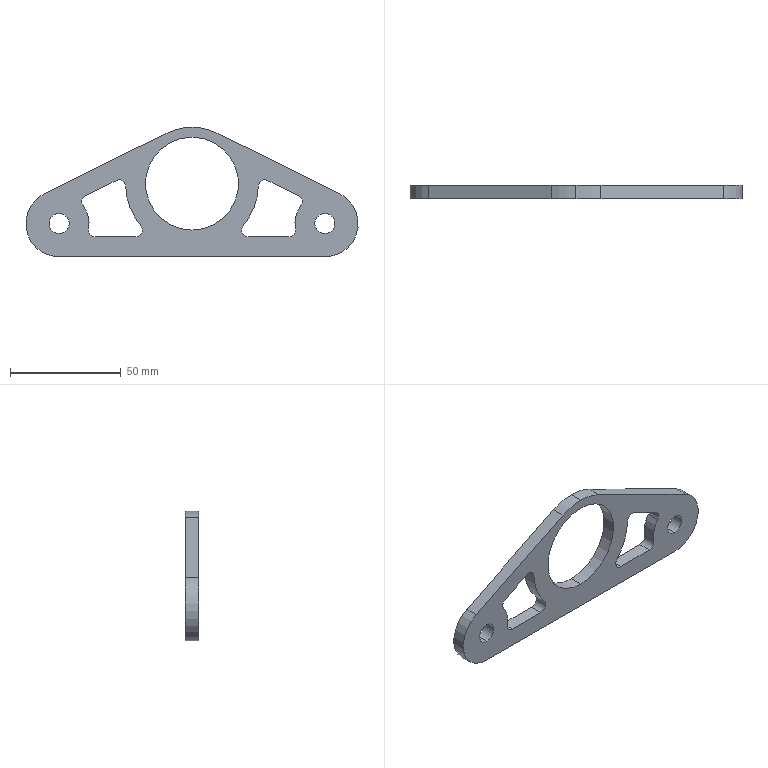Part | STEP file | 2026.6.15-Main Assembly图.sldasm-Part-164 | 1 solid | 33 faces | box 150 x 6 x 58.455 mm | volume 22886 mm3 | cylinder 24 | plane 9 | commonest cylinder face diameters 6 x10 9.06 x4 27.06 x2 30 x2 41.91 x2 50.91 x2
STEP:
#1=CARTESIAN_POINT('',(-1582.519,1443.764,3392.966));
#2=VERTEX_POINT('',#1);
#3=CARTESIAN_POINT('',(-1571.238,1443.764,3395.602));
#4=VERTEX_POINT('',#3);
#5=CARTESIAN_POINT('',(-1571.238,1443.764,3370.147));
#6=DIRECTION('',(0.,1.,0.));
#7=DIRECTION('',(0.,0.,1.));
#8=AXIS2_PLACEMENT_3D('',#5,#6,#7);
#9=CIRCLE('',#8,25.455);
#10=EDGE_CURVE('',#2,#4,#9,.T.);
#11=ORIENTED_EDGE('',*,*,#10,.F.);
#12=CARTESIAN_POINT('',(-1637.886,1443.764,3365.593));
#13=VERTEX_POINT('',#12);
#14=CARTESIAN_POINT('',(-1637.886,1443.764,3365.593));
#15=DIRECTION('',(-0.8964,0.,-0.4432));
#16=VECTOR('',#15,1000.);
#17=LINE('',#14,#16);
#18=EDGE_CURVE('',#2,#13,#17,.T.);
#19=ORIENTED_EDGE('',*,*,#18,.T.);
#20=CARTESIAN_POINT('',(-1631.238,1443.764,3337.147));
#21=VERTEX_POINT('',#20);
#22=CARTESIAN_POINT('',(-1631.238,1443.764,3352.147));
#23=DIRECTION('',(0.,1.,0.));
#24=DIRECTION('',(0.,0.,1.));
#25=AXIS2_PLACEMENT_3D('',#22,#23,#24);
#26=CIRCLE('',#25,15.);
#27=EDGE_CURVE('',#21,#13,#26,.T.);
#28=ORIENTED_EDGE('',*,*,#27,.F.);
#29=CARTESIAN_POINT('',(-1511.238,1443.764,3337.147));
#30=VERTEX_POINT('',#29);
#31=CARTESIAN_POINT('',(-1631.238,1443.764,3337.147));
#32=DIRECTION('',(1.,0.,0.));
#33=VECTOR('',#32,1000.);
#34=LINE('',#31,#33);
#35=EDGE_CURVE('',#21,#30,#34,.T.);
#36=ORIENTED_EDGE('',*,*,#35,.T.);
#37=CARTESIAN_POINT('',(-1504.591,1443.764,3365.593));
#38=VERTEX_POINT('',#37);
#39=CARTESIAN_POINT('',(-1511.238,1443.764,3352.147));
#40=DIRECTION('',(0.,1.,0.));
#41=DIRECTION('',(0.,0.,1.));
#42=AXIS2_PLACEMENT_3D('',#39,#40,#41);
#43=CIRCLE('',#42,15.);
#44=EDGE_CURVE('',#38,#30,#43,.T.);
#45=ORIENTED_EDGE('',*,*,#44,.F.);
#46=CARTESIAN_POINT('',(-1559.957,1443.764,3392.966));
#47=VERTEX_POINT('',#46);
#48=CARTESIAN_POINT('',(-1504.591,1443.764,3365.593));
#49=DIRECTION('',(-0.8964,0.,0.4432));
#50=VECTOR('',#49,1000.);
#51=LINE('',#48,#50);
#52=EDGE_CURVE('',#38,#47,#51,.T.);
#53=ORIENTED_EDGE('',*,*,#52,.T.);
#54=CARTESIAN_POINT('',(-1571.238,1443.764,3370.147));
#55=DIRECTION('',(0.,1.,0.));
#56=DIRECTION('',(0.,0.,1.));
#57=AXIS2_PLACEMENT_3D('',#54,#55,#56);
#58=CIRCLE('',#57,25.455);
#59=EDGE_CURVE('',#4,#47,#58,.T.);
#60=ORIENTED_EDGE('',*,*,#59,.F.);
#61=EDGE_LOOP('',(#11,#19,#28,#36,#45,#53,#60));
#62=FACE_OUTER_BOUND('',#61,.T.);
#63=CARTESIAN_POINT('',(-1631.238,1443.764,3356.677));
#64=VERTEX_POINT('',#63);
#65=CARTESIAN_POINT('',(-1631.238,1443.764,3347.617));
#66=VERTEX_POINT('',#65);
#67=CARTESIAN_POINT('',(-1631.238,1443.764,3352.147));
#68=DIRECTION('',(0.,1.,0.));
#69=DIRECTION('',(0.,0.,1.));
#70=AXIS2_PLACEMENT_3D('',#67,#68,#69);
#71=CIRCLE('',#70,4.53);
#72=EDGE_CURVE('',#64,#66,#71,.T.);
#73=ORIENTED_EDGE('',*,*,#72,.T.);
#74=CARTESIAN_POINT('',(-1631.238,1443.764,3352.147));
#75=DIRECTION('',(0.,1.,0.));
#76=DIRECTION('',(0.,0.,1.));
#77=AXIS2_PLACEMENT_3D('',#74,#75,#76);
#78=CIRCLE('',#77,4.53);
#79=EDGE_CURVE('',#66,#64,#78,.T.);
#80=ORIENTED_EDGE('',*,*,#79,.T.);
#81=EDGE_LOOP('',(#73,#80));
#82=FACE_BOUND('',#81,.T.);
#83=CARTESIAN_POINT('',(-1511.238,1443.764,3356.677));
#84=VERTEX_POINT('',#83);
#85=CARTESIAN_POINT('',(-1511.238,1443.764,3347.617));
#86=VERTEX_POINT('',#85);
#87=CARTESIAN_POINT('',(-1511.238,1443.764,3352.147));
#88=DIRECTION('',(0.,1.,0.));
#89=DIRECTION('',(0.,0.,1.));
#90=AXIS2_PLACEMENT_3D('',#87,#88,#89);
#91=CIRCLE('',#90,4.53);
#92=EDGE_CURVE('',#84,#86,#91,.T.);
#93=ORIENTED_EDGE('',*,*,#92,.T.);
#94=CARTESIAN_POINT('',(-1511.238,1443.764,3352.147));
#95=DIRECTION('',(0.,1.,0.));
#96=DIRECTION('',(0.,0.,1.));
#97=AXIS2_PLACEMENT_3D('',#94,#95,#96);
#98=CIRCLE('',#97,4.53);
#99=EDGE_CURVE('',#86,#84,#98,.T.);
#100=ORIENTED_EDGE('',*,*,#99,.T.);
#101=EDGE_LOOP('',(#93,#100));
#102=FACE_BOUND('',#101,.T.);
#103=CARTESIAN_POINT('',(-1571.238,1443.764,3391.102));
#104=VERTEX_POINT('',#103);
#105=CARTESIAN_POINT('',(-1571.238,1443.764,3349.192));
#106=VERTEX_POINT('',#105);
#107=CARTESIAN_POINT('',(-1571.238,1443.764,3370.147));
#108=DIRECTION('',(0.,1.,0.));
#109=DIRECTION('',(0.,0.,1.));
#110=AXIS2_PLACEMENT_3D('',#107,#108,#109);
#111=CIRCLE('',#110,20.955);
#112=EDGE_CURVE('',#104,#106,#111,.T.);
#113=ORIENTED_EDGE('',*,*,#112,.T.);
#114=CARTESIAN_POINT('',(-1571.238,1443.764,3370.147));
#115=DIRECTION('',(0.,1.,0.));
#116=DIRECTION('',(0.,0.,1.));
#117=AXIS2_PLACEMENT_3D('',#114,#115,#116);
#118=CIRCLE('',#117,20.955);
#119=EDGE_CURVE('',#106,#104,#118,.T.);
#120=ORIENTED_EDGE('',*,*,#119,.T.);
#121=EDGE_LOOP('',(#113,#120));
#122=FACE_BOUND('',#121,.T.);
#123=CARTESIAN_POINT('',(-1523.151,1443.764,3364.73));
#124=VERTEX_POINT('',#123);
#125=CARTESIAN_POINT('',(-1536.978,1443.764,3371.565));
#126=VERTEX_POINT('',#125);
#127=CARTESIAN_POINT('',(-1536.978,1443.764,3371.565));
#128=DIRECTION('',(-0.8964,0.,0.4432));
#129=VECTOR('',#128,1000.);
#130=LINE('',#127,#129);
#131=EDGE_CURVE('',#124,#126,#130,.T.);
#132=ORIENTED_EDGE('',*,*,#131,.F.);
#133=CARTESIAN_POINT('',(-1522.077,1443.764,3360.245));
#134=VERTEX_POINT('',#133);
#135=CARTESIAN_POINT('',(-1524.481,1443.764,3362.04));
#136=DIRECTION('',(0.,1.,0.));
#137=DIRECTION('',(0.,0.,1.));
#138=AXIS2_PLACEMENT_3D('',#135,#136,#137);
#139=CIRCLE('',#138,3.);
#140=EDGE_CURVE('',#124,#134,#139,.T.);
#141=ORIENTED_EDGE('',*,*,#140,.T.);
#142=CARTESIAN_POINT('',(-1524.544,1443.764,3349.691));
#143=VERTEX_POINT('',#142);
#144=CARTESIAN_POINT('',(-1511.238,1443.764,3352.147));
#145=DIRECTION('',(0.,1.,0.));
#146=DIRECTION('',(0.,0.,1.));
#147=AXIS2_PLACEMENT_3D('',#144,#145,#146);
#148=CIRCLE('',#147,13.53);
#149=EDGE_CURVE('',#143,#134,#148,.T.);
#150=ORIENTED_EDGE('',*,*,#149,.F.);
#151=CARTESIAN_POINT('',(-1527.494,1443.764,3346.147));
#152=VERTEX_POINT('',#151);
#153=CARTESIAN_POINT('',(-1527.494,1443.764,3349.147));
#154=DIRECTION('',(0.,1.,0.));
#155=DIRECTION('',(0.,0.,1.));
#156=AXIS2_PLACEMENT_3D('',#153,#154,#155);
#157=CIRCLE('',#156,3.);
#158=EDGE_CURVE('',#143,#152,#157,.T.);
#159=ORIENTED_EDGE('',*,*,#158,.T.);
#160=CARTESIAN_POINT('',(-1545.841,1443.764,3346.147));
#161=VERTEX_POINT('',#160);
#162=CARTESIAN_POINT('',(-1527.494,1443.764,3346.147));
#163=DIRECTION('',(1.,0.,0.));
#164=VECTOR('',#163,1000.);
#165=LINE('',#162,#164);
#166=EDGE_CURVE('',#161,#152,#165,.T.);
#167=ORIENTED_EDGE('',*,*,#166,.F.);
#168=CARTESIAN_POINT('',(-1548.153,1443.764,3351.059));
#169=VERTEX_POINT('',#168);
#170=CARTESIAN_POINT('',(-1545.841,1443.764,3349.147));
#171=DIRECTION('',(0.,1.,0.));
#172=DIRECTION('',(0.,0.,1.));
#173=AXIS2_PLACEMENT_3D('',#170,#171,#172);
#174=CIRCLE('',#173,3.);
#175=EDGE_CURVE('',#161,#169,#174,.T.);
#176=ORIENTED_EDGE('',*,*,#175,.T.);
#177=CARTESIAN_POINT('',(-1541.306,1443.764,3368.992));
#178=VERTEX_POINT('',#177);
#179=CARTESIAN_POINT('',(-1571.238,1443.764,3370.147));
#180=DIRECTION('',(0.,1.,0.));
#181=DIRECTION('',(0.,0.,1.));
#182=AXIS2_PLACEMENT_3D('',#179,#180,#181);
#183=CIRCLE('',#182,29.955);
#184=EDGE_CURVE('',#178,#169,#183,.T.);
#185=ORIENTED_EDGE('',*,*,#184,.F.);
#186=CARTESIAN_POINT('',(-1538.308,1443.764,3371.876));
#187=VERTEX_POINT('',#186);
#188=CARTESIAN_POINT('',(-1538.308,1443.764,3368.876));
#189=DIRECTION('',(0.,1.,0.));
#190=DIRECTION('',(0.,0.,1.));
#191=AXIS2_PLACEMENT_3D('',#188,#189,#190);
#192=CIRCLE('',#191,3.);
#193=EDGE_CURVE('',#178,#187,#192,.T.);
#194=ORIENTED_EDGE('',*,*,#193,.T.);
#195=CARTESIAN_POINT('',(-1538.308,1443.764,3368.876));
#196=DIRECTION('',(0.,1.,0.));
#197=DIRECTION('',(0.,0.,1.));
#198=AXIS2_PLACEMENT_3D('',#195,#196,#197);
#199=CIRCLE('',#198,3.);
#200=EDGE_CURVE('',#187,#126,#199,.T.);
#201=ORIENTED_EDGE('',*,*,#200,.T.);
#202=EDGE_LOOP('',(#132,#141,#150,#159,#167,#176,#185,#194,#201));
#203=FACE_BOUND('',#202,.T.);
#204=CARTESIAN_POINT('',(-1594.324,1443.764,3351.059));
#205=VERTEX_POINT('',#204);
#206=CARTESIAN_POINT('',(-1596.636,1443.764,3346.147));
#207=VERTEX_POINT('',#206);
#208=CARTESIAN_POINT('',(-1596.636,1443.764,3349.147));
#209=DIRECTION('',(0.,1.,0.));
#210=DIRECTION('',(0.,0.,1.));
#211=AXIS2_PLACEMENT_3D('',#208,#209,#210);
#212=CIRCLE('',#211,3.);
#213=EDGE_CURVE('',#205,#207,#212,.T.);
#214=ORIENTED_EDGE('',*,*,#213,.T.);
#215=CARTESIAN_POINT('',(-1614.983,1443.764,3346.147));
#216=VERTEX_POINT('',#215);
#217=CARTESIAN_POINT('',(-1614.983,1443.764,3346.147));
#218=DIRECTION('',(1.,0.,0.));
#219=VECTOR('',#218,1000.);
#220=LINE('',#217,#219);
#221=EDGE_CURVE('',#216,#207,#220,.T.);
#222=ORIENTED_EDGE('',*,*,#221,.F.);
#223=CARTESIAN_POINT('',(-1617.933,1443.764,3349.691));
#224=VERTEX_POINT('',#223);
#225=CARTESIAN_POINT('',(-1614.983,1443.764,3349.147));
#226=DIRECTION('',(0.,1.,0.));
#227=DIRECTION('',(0.,0.,1.));
#228=AXIS2_PLACEMENT_3D('',#225,#226,#227);
#229=CIRCLE('',#228,3.);
#230=EDGE_CURVE('',#216,#224,#229,.T.);
#231=ORIENTED_EDGE('',*,*,#230,.T.);
#232=CARTESIAN_POINT('',(-1620.399,1443.764,3360.245));
#233=VERTEX_POINT('',#232);
#234=CARTESIAN_POINT('',(-1631.238,1443.764,3352.147));
#235=DIRECTION('',(0.,1.,0.));
#236=DIRECTION('',(0.,0.,1.));
#237=AXIS2_PLACEMENT_3D('',#234,#235,#236);
#238=CIRCLE('',#237,13.53);
#239=EDGE_CURVE('',#233,#224,#238,.T.);
#240=ORIENTED_EDGE('',*,*,#239,.F.);
#241=CARTESIAN_POINT('',(-1619.325,1443.764,3364.73));
#242=VERTEX_POINT('',#241);
#243=CARTESIAN_POINT('',(-1617.996,1443.764,3362.04));
#244=DIRECTION('',(0.,1.,0.));
#245=DIRECTION('',(0.,0.,1.));
#246=AXIS2_PLACEMENT_3D('',#243,#244,#245);
#247=CIRCLE('',#246,3.);
#248=EDGE_CURVE('',#233,#242,#247,.T.);
#249=ORIENTED_EDGE('',*,*,#248,.T.);
#250=CARTESIAN_POINT('',(-1605.498,1443.764,3371.565));
#251=VERTEX_POINT('',#250);
#252=CARTESIAN_POINT('',(-1605.498,1443.764,3371.565));
#253=DIRECTION('',(-0.8964,0.,-0.4432));
#254=VECTOR('',#253,1000.);
#255=LINE('',#252,#254);
#256=EDGE_CURVE('',#251,#242,#255,.T.);
#257=ORIENTED_EDGE('',*,*,#256,.F.);
#258=CARTESIAN_POINT('',(-1604.169,1443.764,3371.876));
#259=VERTEX_POINT('',#258);
#260=CARTESIAN_POINT('',(-1604.169,1443.764,3368.876));
#261=DIRECTION('',(0.,1.,0.));
#262=DIRECTION('',(0.,0.,1.));
#263=AXIS2_PLACEMENT_3D('',#260,#261,#262);
#264=CIRCLE('',#263,3.);
#265=EDGE_CURVE('',#251,#259,#264,.T.);
#266=ORIENTED_EDGE('',*,*,#265,.T.);
#267=CARTESIAN_POINT('',(-1601.171,1443.764,3368.992));
#268=VERTEX_POINT('',#267);
#269=CARTESIAN_POINT('',(-1604.169,1443.764,3368.876));
#270=DIRECTION('',(0.,1.,0.));
#271=DIRECTION('',(0.,0.,1.));
#272=AXIS2_PLACEMENT_3D('',#269,#270,#271);
#273=CIRCLE('',#272,3.);
#274=EDGE_CURVE('',#259,#268,#273,.T.);
#275=ORIENTED_EDGE('',*,*,#274,.T.);
#276=CARTESIAN_POINT('',(-1571.238,1443.764,3370.147));
#277=DIRECTION('',(0.,1.,0.));
#278=DIRECTION('',(0.,0.,1.));
#279=AXIS2_PLACEMENT_3D('',#276,#277,#278);
#280=CIRCLE('',#279,29.955);
#281=EDGE_CURVE('',#205,#268,#280,.T.);
#282=ORIENTED_EDGE('',*,*,#281,.F.);
#283=EDGE_LOOP('',(#214,#222,#231,#240,#249,#257,#266,#275,#282));
#284=FACE_BOUND('',#283,.T.);
#285=CARTESIAN_POINT('',(-1631.238,1443.764,3352.147));
#286=DIRECTION('',(0.,-1.,0.));
#287=DIRECTION('',(-1.,0.,0.));
#288=AXIS2_PLACEMENT_3D('',#285,#286,#287);
#289=PLANE('',#288);
#290=ADVANCED_FACE('',(#62,#82,#102,#122,#203,#284),#289,.T.);
#291=CARTESIAN_POINT('',(-1527.494,1449.764,3346.147));
#292=VERTEX_POINT('',#291);
#293=CARTESIAN_POINT('',(-1545.841,1449.764,3346.147));
#294=VERTEX_POINT('',#293);
#295=CARTESIAN_POINT('',(-1631.238,1449.764,3346.147));
#296=DIRECTION('',(-1.,0.,0.));
#297=VECTOR('',#296,1000.);
#298=LINE('',#295,#297);
#299=EDGE_CURVE('',#292,#294,#298,.T.);
#300=ORIENTED_EDGE('',*,*,#299,.T.);
#301=CARTESIAN_POINT('',(-1545.841,1449.764,3346.147));
#302=DIRECTION('',(0.,-1.,0.));
#303=VECTOR('',#302,1000.);
#304=LINE('',#301,#303);
#305=EDGE_CURVE('',#294,#161,#304,.T.);
#306=ORIENTED_EDGE('',*,*,#305,.T.);
#307=ORIENTED_EDGE('',*,*,#166,.T.);
#308=CARTESIAN_POINT('',(-1527.494,1449.764,3346.147));
#309=DIRECTION('',(0.,1.,0.));
#310=VECTOR('',#309,1000.);
#311=LINE('',#308,#310);
#312=EDGE_CURVE('',#152,#292,#311,.T.);
#313=ORIENTED_EDGE('',*,*,#312,.T.);
#314=EDGE_LOOP('',(#300,#306,#307,#313));
#315=FACE_OUTER_BOUND('',#314,.T.);
#316=CARTESIAN_POINT('',(-1527.494,1449.764,3346.147));
#317=DIRECTION('',(0.,0.,1.));
#318=DIRECTION('',(-1.,0.,0.));
#319=AXIS2_PLACEMENT_3D('',#316,#317,#318);
#320=PLANE('',#319);
#321=ADVANCED_FACE('',(#315),#320,.T.);
#322=ORIENTED_EDGE('',*,*,#305,.F.);
#323=CARTESIAN_POINT('',(-1548.153,1449.764,3351.059));
#324=VERTEX_POINT('',#323);
#325=CARTESIAN_POINT('',(-1545.841,1449.764,3349.147));
#326=DIRECTION('',(0.,1.,0.));
#327=DIRECTION('',(0.,0.,1.));
#328=AXIS2_PLACEMENT_3D('',#325,#326,#327);
#329=CIRCLE('',#328,3.);
#330=EDGE_CURVE('',#294,#324,#329,.T.);
#331=ORIENTED_EDGE('',*,*,#330,.T.);
#332=CARTESIAN_POINT('',(-1548.153,1449.764,3351.059));
#333=DIRECTION('',(0.,1.,0.));
#334=VECTOR('',#333,1000.);
#335=LINE('',#332,#334);
#336=EDGE_CURVE('',#169,#324,#335,.T.);
#337=ORIENTED_EDGE('',*,*,#336,.F.);
#338=ORIENTED_EDGE('',*,*,#175,.F.);
#339=EDGE_LOOP('',(#322,#331,#337,#338));
#340=FACE_OUTER_BOUND('',#339,.T.);
#341=CARTESIAN_POINT('',(-1545.841,1449.764,3349.147));
#342=DIRECTION('',(0.,-1.,0.));
#343=DIRECTION('',(0.,0.,-1.));
#344=AXIS2_PLACEMENT_3D('',#341,#342,#343);
#345=CYLINDRICAL_SURFACE('',#344,3.);
#346=ADVANCED_FACE('',(#340),#345,.F.);
#347=CARTESIAN_POINT('',(-1541.306,1449.764,3368.992));
#348=VERTEX_POINT('',#347);
#349=CARTESIAN_POINT('',(-1571.238,1449.764,3370.147));
#350=DIRECTION('',(0.,-1.,0.));
#351=DIRECTION('',(0.,0.,1.));
#352=AXIS2_PLACEMENT_3D('',#349,#350,#351);
#353=CIRCLE('',#352,29.955);
#354=EDGE_CURVE('',#324,#348,#353,.T.);
#355=ORIENTED_EDGE('',*,*,#354,.T.);
#356=CARTESIAN_POINT('',(-1541.306,1449.764,3368.992));
#357=DIRECTION('',(0.,-1.,0.));
#358=VECTOR('',#357,1000.);
#359=LINE('',#356,#358);
#360=EDGE_CURVE('',#348,#178,#359,.T.);
#361=ORIENTED_EDGE('',*,*,#360,.T.);
#362=ORIENTED_EDGE('',*,*,#184,.T.);
#363=ORIENTED_EDGE('',*,*,#336,.T.);
#364=EDGE_LOOP('',(#355,#361,#362,#363));
#365=FACE_OUTER_BOUND('',#364,.T.);
#366=CARTESIAN_POINT('',(-1571.238,1449.764,3370.147));
#367=DIRECTION('',(0.,-1.,0.));
#368=DIRECTION('',(0.,0.,-1.));
#369=AXIS2_PLACEMENT_3D('',#366,#367,#368);
#370=CYLINDRICAL_SURFACE('',#369,29.955);
#371=ADVANCED_FACE('',(#365),#370,.T.);
#372=CARTESIAN_POINT('',(-1538.308,1449.764,3371.876));
#373=VERTEX_POINT('',#372);
#374=CARTESIAN_POINT('',(-1538.308,1449.764,3371.876));
#375=DIRECTION('',(0.,-1.,0.));
#376=VECTOR('',#375,1000.);
#377=LINE('',#374,#376);
#378=EDGE_CURVE('',#373,#187,#377,.T.);
#379=ORIENTED_EDGE('',*,*,#378,.F.);
#380=CARTESIAN_POINT('',(-1536.978,1449.764,3371.565));
#381=VERTEX_POINT('',#380);
#382=CARTESIAN_POINT('',(-1538.308,1449.764,3368.876));
#383=DIRECTION('',(0.,1.,0.));
#384=DIRECTION('',(0.,0.,1.));
#385=AXIS2_PLACEMENT_3D('',#382,#383,#384);
#386=CIRCLE('',#385,3.);
#387=EDGE_CURVE('',#373,#381,#386,.T.);
#388=ORIENTED_EDGE('',*,*,#387,.T.);
#389=CARTESIAN_POINT('',(-1536.978,1449.764,3371.565));
#390=DIRECTION('',(0.,1.,0.));
#391=VECTOR('',#390,1000.);
#392=LINE('',#389,#391);
#393=EDGE_CURVE('',#126,#381,#392,.T.);
#394=ORIENTED_EDGE('',*,*,#393,.F.);
#395=ORIENTED_EDGE('',*,*,#200,.F.);
#396=EDGE_LOOP('',(#379,#388,#394,#395));
#397=FACE_OUTER_BOUND('',#396,.T.);
#398=CARTESIAN_POINT('',(-1538.308,1449.764,3368.876));
#399=DIRECTION('',(0.,-1.,0.));
#400=DIRECTION('',(0.,0.,-1.));
#401=AXIS2_PLACEMENT_3D('',#398,#399,#400);
#402=CYLINDRICAL_SURFACE('',#401,3.);
#403=ADVANCED_FACE('',(#397),#402,.F.);
#404=CARTESIAN_POINT('',(-1523.151,1449.764,3364.73));
#405=VERTEX_POINT('',#404);
#406=CARTESIAN_POINT('',(-1536.978,1449.764,3371.565));
#407=DIRECTION('',(0.8964,0.,-0.4432));
#408=VECTOR('',#407,1000.);
#409=LINE('',#406,#408);
#410=EDGE_CURVE('',#381,#405,#409,.T.);
#411=ORIENTED_EDGE('',*,*,#410,.T.);
#412=CARTESIAN_POINT('',(-1523.151,1449.764,3364.73));
#413=DIRECTION('',(0.,-1.,0.));
#414=VECTOR('',#413,1000.);
#415=LINE('',#412,#414);
#416=EDGE_CURVE('',#405,#124,#415,.T.);
#417=ORIENTED_EDGE('',*,*,#416,.T.);
#418=ORIENTED_EDGE('',*,*,#131,.T.);
#419=ORIENTED_EDGE('',*,*,#393,.T.);
#420=EDGE_LOOP('',(#411,#417,#418,#419));
#421=FACE_OUTER_BOUND('',#420,.T.);
#422=CARTESIAN_POINT('',(-1536.978,1449.764,3371.565));
#423=DIRECTION('',(-0.4432,0.,-0.8964));
#424=DIRECTION('',(0.,1.,0.));
#425=AXIS2_PLACEMENT_3D('',#422,#423,#424);
#426=PLANE('',#425);
#427=ADVANCED_FACE('',(#421),#426,.T.);
#428=ORIENTED_EDGE('',*,*,#416,.F.);
#429=CARTESIAN_POINT('',(-1522.077,1449.764,3360.245));
#430=VERTEX_POINT('',#429);
#431=CARTESIAN_POINT('',(-1524.481,1449.764,3362.04));
#432=DIRECTION('',(0.,1.,0.));
#433=DIRECTION('',(0.,0.,1.));
#434=AXIS2_PLACEMENT_3D('',#431,#432,#433);
#435=CIRCLE('',#434,3.);
#436=EDGE_CURVE('',#405,#430,#435,.T.);
#437=ORIENTED_EDGE('',*,*,#436,.T.);
#438=CARTESIAN_POINT('',(-1522.077,1449.764,3360.245));
#439=DIRECTION('',(0.,1.,0.));
#440=VECTOR('',#439,1000.);
#441=LINE('',#438,#440);
#442=EDGE_CURVE('',#134,#430,#441,.T.);
#443=ORIENTED_EDGE('',*,*,#442,.F.);
#444=ORIENTED_EDGE('',*,*,#140,.F.);
#445=EDGE_LOOP('',(#428,#437,#443,#444));
#446=FACE_OUTER_BOUND('',#445,.T.);
#447=CARTESIAN_POINT('',(-1524.481,1449.764,3362.04));
#448=DIRECTION('',(0.,-1.,0.));
#449=DIRECTION('',(0.,0.,-1.));
#450=AXIS2_PLACEMENT_3D('',#447,#448,#449);
#451=CYLINDRICAL_SURFACE('',#450,3.);
#452=ADVANCED_FACE('',(#446),#451,.F.);
#453=CARTESIAN_POINT('',(-1524.544,1449.764,3349.691));
#454=VERTEX_POINT('',#453);
#455=CARTESIAN_POINT('',(-1511.238,1449.764,3352.147));
#456=DIRECTION('',(0.,-1.,0.));
#457=DIRECTION('',(0.,0.,1.));
#458=AXIS2_PLACEMENT_3D('',#455,#456,#457);
#459=CIRCLE('',#458,13.53);
#460=EDGE_CURVE('',#430,#454,#459,.T.);
#461=ORIENTED_EDGE('',*,*,#460,.T.);
#462=CARTESIAN_POINT('',(-1524.544,1449.764,3349.691));
#463=DIRECTION('',(0.,-1.,0.));
#464=VECTOR('',#463,1000.);
#465=LINE('',#462,#464);
#466=EDGE_CURVE('',#454,#143,#465,.T.);
#467=ORIENTED_EDGE('',*,*,#466,.T.);
#468=ORIENTED_EDGE('',*,*,#149,.T.);
#469=ORIENTED_EDGE('',*,*,#442,.T.);
#470=EDGE_LOOP('',(#461,#467,#468,#469));
#471=FACE_OUTER_BOUND('',#470,.T.);
#472=CARTESIAN_POINT('',(-1511.238,1449.764,3352.147));
#473=DIRECTION('',(0.,-1.,0.));
#474=DIRECTION('',(0.,0.,-1.));
#475=AXIS2_PLACEMENT_3D('',#472,#473,#474);
#476=CYLINDRICAL_SURFACE('',#475,13.53);
#477=ADVANCED_FACE('',(#471),#476,.T.);
#478=ORIENTED_EDGE('',*,*,#466,.F.);
#479=CARTESIAN_POINT('',(-1527.494,1449.764,3349.147));
#480=DIRECTION('',(0.,1.,0.));
#481=DIRECTION('',(0.,0.,1.));
#482=AXIS2_PLACEMENT_3D('',#479,#480,#481);
#483=CIRCLE('',#482,3.);
#484=EDGE_CURVE('',#454,#292,#483,.T.);
#485=ORIENTED_EDGE('',*,*,#484,.T.);
#486=ORIENTED_EDGE('',*,*,#312,.F.);
#487=ORIENTED_EDGE('',*,*,#158,.F.);
#488=EDGE_LOOP('',(#478,#485,#486,#487));
#489=FACE_OUTER_BOUND('',#488,.T.);
#490=CARTESIAN_POINT('',(-1527.494,1449.764,3349.147));
#491=DIRECTION('',(0.,-1.,0.));
#492=DIRECTION('',(0.,0.,-1.));
#493=AXIS2_PLACEMENT_3D('',#490,#491,#492);
#494=CYLINDRICAL_SURFACE('',#493,3.);
#495=ADVANCED_FACE('',(#489),#494,.F.);
#496=CARTESIAN_POINT('',(-1631.238,1449.764,3337.147));
#497=VERTEX_POINT('',#496);
#498=CARTESIAN_POINT('',(-1631.238,1449.764,3337.147));
#499=DIRECTION('',(0.,-1.,0.));
#500=VECTOR('',#499,1000.);
#501=LINE('',#498,#500);
#502=EDGE_CURVE('',#497,#21,#501,.T.);
#503=ORIENTED_EDGE('',*,*,#502,.F.);
#504=CARTESIAN_POINT('',(-1511.238,1449.764,3337.147));
#505=VERTEX_POINT('',#504);
#506=CARTESIAN_POINT('',(-1631.238,1449.764,3337.147));
#507=DIRECTION('',(1.,0.,0.));
#508=VECTOR('',#507,1000.);
#509=LINE('',#506,#508);
#510=EDGE_CURVE('',#497,#505,#509,.T.);
#511=ORIENTED_EDGE('',*,*,#510,.T.);
#512=CARTESIAN_POINT('',(-1511.238,1449.764,3337.147));
#513=DIRECTION('',(0.,1.,0.));
#514=VECTOR('',#513,1000.);
#515=LINE('',#512,#514);
#516=EDGE_CURVE('',#30,#505,#515,.T.);
#517=ORIENTED_EDGE('',*,*,#516,.F.);
#518=ORIENTED_EDGE('',*,*,#35,.F.);
#519=EDGE_LOOP('',(#503,#511,#517,#518));
#520=FACE_OUTER_BOUND('',#519,.T.);
#521=CARTESIAN_POINT('',(-1631.238,1449.764,3337.147));
#522=DIRECTION('',(0.,0.,1.));
#523=DIRECTION('',(-1.,0.,0.));
#524=AXIS2_PLACEMENT_3D('',#521,#522,#523);
#525=PLANE('',#524);
#526=ADVANCED_FACE('',(#520),#525,.F.);
#527=CARTESIAN_POINT('',(-1504.591,1449.764,3365.593));
#528=VERTEX_POINT('',#527);
#529=CARTESIAN_POINT('',(-1511.238,1449.764,3352.147));
#530=DIRECTION('',(0.,-1.,0.));
#531=DIRECTION('',(0.,0.,1.));
#532=AXIS2_PLACEMENT_3D('',#529,#530,#531);
#533=CIRCLE('',#532,15.);
#534=EDGE_CURVE('',#505,#528,#533,.T.);
#535=ORIENTED_EDGE('',*,*,#534,.T.);
#536=CARTESIAN_POINT('',(-1504.591,1449.764,3365.593));
#537=DIRECTION('',(0.,-1.,0.));
#538=VECTOR('',#537,1000.);
#539=LINE('',#536,#538);
#540=EDGE_CURVE('',#528,#38,#539,.T.);
#541=ORIENTED_EDGE('',*,*,#540,.T.);
#542=ORIENTED_EDGE('',*,*,#44,.T.);
#543=ORIENTED_EDGE('',*,*,#516,.T.);
#544=EDGE_LOOP('',(#535,#541,#542,#543));
#545=FACE_OUTER_BOUND('',#544,.T.);
#546=CARTESIAN_POINT('',(-1511.238,1449.764,3352.147));
#547=DIRECTION('',(0.,-1.,0.));
#548=DIRECTION('',(0.,0.,-1.));
#549=AXIS2_PLACEMENT_3D('',#546,#547,#548);
#550=CYLINDRICAL_SURFACE('',#549,15.);
#551=ADVANCED_FACE('',(#545),#550,.T.);
#552=ORIENTED_EDGE('',*,*,#540,.F.);
#553=CARTESIAN_POINT('',(-1559.957,1449.764,3392.966));
#554=VERTEX_POINT('',#553);
#555=CARTESIAN_POINT('',(-1504.591,1449.764,3365.593));
#556=DIRECTION('',(-0.8964,0.,0.4432));
#557=VECTOR('',#556,1000.);
#558=LINE('',#555,#557);
#559=EDGE_CURVE('',#528,#554,#558,.T.);
#560=ORIENTED_EDGE('',*,*,#559,.T.);
#561=CARTESIAN_POINT('',(-1559.957,1449.764,3392.966));
#562=DIRECTION('',(0.,1.,0.));
#563=VECTOR('',#562,1000.);
#564=LINE('',#561,#563);
#565=EDGE_CURVE('',#47,#554,#564,.T.);
#566=ORIENTED_EDGE('',*,*,#565,.F.);
#567=ORIENTED_EDGE('',*,*,#52,.F.);
#568=EDGE_LOOP('',(#552,#560,#566,#567));
#569=FACE_OUTER_BOUND('',#568,.T.);
#570=CARTESIAN_POINT('',(-1504.591,1449.764,3365.593));
#571=DIRECTION('',(-0.4432,0.,-0.8964));
#572=DIRECTION('',(0.,1.,0.));
#573=AXIS2_PLACEMENT_3D('',#570,#571,#572);
#574=PLANE('',#573);
#575=ADVANCED_FACE('',(#569),#574,.F.);
#576=CARTESIAN_POINT('',(-1571.238,1449.764,3395.602));
#577=VERTEX_POINT('',#576);
#578=CARTESIAN_POINT('',(-1571.238,1449.764,3395.602));
#579=DIRECTION('',(0.,-1.,0.));
#580=VECTOR('',#579,1000.);
#581=LINE('',#578,#580);
#582=EDGE_CURVE('',#577,#4,#581,.T.);
#583=ORIENTED_EDGE('',*,*,#582,.F.);
#584=CARTESIAN_POINT('',(-1582.519,1449.764,3392.966));
#585=VERTEX_POINT('',#584);
#586=CARTESIAN_POINT('',(-1571.238,1449.764,3370.147));
#587=DIRECTION('',(0.,-1.,0.));
#588=DIRECTION('',(0.,0.,1.));
#589=AXIS2_PLACEMENT_3D('',#586,#587,#588);
#590=CIRCLE('',#589,25.455);
#591=EDGE_CURVE('',#577,#585,#590,.T.);
#592=ORIENTED_EDGE('',*,*,#591,.T.);
#593=CARTESIAN_POINT('',(-1582.519,1449.764,3392.966));
#594=DIRECTION('',(0.,-1.,0.));
#595=VECTOR('',#594,1000.);
#596=LINE('',#593,#595);
#597=EDGE_CURVE('',#585,#2,#596,.T.);
#598=ORIENTED_EDGE('',*,*,#597,.T.);
#599=ORIENTED_EDGE('',*,*,#10,.T.);
#600=EDGE_LOOP('',(#583,#592,#598,#599));
#601=FACE_OUTER_BOUND('',#600,.T.);
#602=CARTESIAN_POINT('',(-1571.238,1449.764,3370.147));
#603=DIRECTION('',(0.,-1.,0.));
#604=DIRECTION('',(0.,0.,-1.));
#605=AXIS2_PLACEMENT_3D('',#602,#603,#604);
#606=CYLINDRICAL_SURFACE('',#605,25.455);
#607=ADVANCED_FACE('',(#601),#606,.T.);
#608=ORIENTED_EDGE('',*,*,#597,.F.);
#609=CARTESIAN_POINT('',(-1637.886,1449.764,3365.593));
#610=VERTEX_POINT('',#609);
#611=CARTESIAN_POINT('',(-1582.519,1449.764,3392.966));
#612=DIRECTION('',(-0.8964,0.,-0.4432));
#613=VECTOR('',#612,1000.);
#614=LINE('',#611,#613);
#615=EDGE_CURVE('',#585,#610,#614,.T.);
#616=ORIENTED_EDGE('',*,*,#615,.T.);
#617=CARTESIAN_POINT('',(-1637.886,1449.764,3365.593));
#618=DIRECTION('',(0.,1.,0.));
#619=VECTOR('',#618,1000.);
#620=LINE('',#617,#619);
#621=EDGE_CURVE('',#13,#610,#620,.T.);
#622=ORIENTED_EDGE('',*,*,#621,.F.);
#623=ORIENTED_EDGE('',*,*,#18,.F.);
#624=EDGE_LOOP('',(#608,#616,#622,#623));
#625=FACE_OUTER_BOUND('',#624,.T.);
#626=CARTESIAN_POINT('',(-1637.886,1449.764,3365.593));
#627=DIRECTION('',(0.4432,0.,-0.8964));
#628=DIRECTION('',(0.,-1.,0.));
#629=AXIS2_PLACEMENT_3D('',#626,#627,#628);
#630=PLANE('',#629);
#631=ADVANCED_FACE('',(#625),#630,.F.);
#632=CARTESIAN_POINT('',(-1631.238,1449.764,3352.147));
#633=DIRECTION('',(0.,-1.,0.));
#634=DIRECTION('',(0.,0.,1.));
#635=AXIS2_PLACEMENT_3D('',#632,#633,#634);
#636=CIRCLE('',#635,15.);
#637=EDGE_CURVE('',#610,#497,#636,.T.);
#638=ORIENTED_EDGE('',*,*,#637,.T.);
#639=ORIENTED_EDGE('',*,*,#502,.T.);
#640=ORIENTED_EDGE('',*,*,#27,.T.);
#641=ORIENTED_EDGE('',*,*,#621,.T.);
#642=EDGE_LOOP('',(#638,#639,#640,#641));
#643=FACE_OUTER_BOUND('',#642,.T.);
#644=CARTESIAN_POINT('',(-1631.238,1449.764,3352.147));
#645=DIRECTION('',(0.,-1.,0.));
#646=DIRECTION('',(0.,0.,-1.));
#647=AXIS2_PLACEMENT_3D('',#644,#645,#646);
#648=CYLINDRICAL_SURFACE('',#647,15.);
#649=ADVANCED_FACE('',(#643),#648,.T.);
#650=CARTESIAN_POINT('',(-1511.238,1449.764,3347.617));
#651=VERTEX_POINT('',#650);
#652=CARTESIAN_POINT('',(-1511.238,1449.764,3347.617));
#653=DIRECTION('',(0.,1.,0.));
#654=VECTOR('',#653,1000.);
#655=LINE('',#652,#654);
#656=EDGE_CURVE('',#86,#651,#655,.T.);
#657=ORIENTED_EDGE('',*,*,#656,.T.);
#658=CARTESIAN_POINT('',(-1511.238,1449.764,3356.677));
#659=VERTEX_POINT('',#658);
#660=CARTESIAN_POINT('',(-1511.238,1449.764,3352.147));
#661=DIRECTION('',(0.,1.,0.));
#662=DIRECTION('',(0.,0.,1.));
#663=AXIS2_PLACEMENT_3D('',#660,#661,#662);
#664=CIRCLE('',#663,4.53);
#665=EDGE_CURVE('',#651,#659,#664,.T.);
#666=ORIENTED_EDGE('',*,*,#665,.T.);
#667=CARTESIAN_POINT('',(-1511.238,1449.764,3356.677));
#668=DIRECTION('',(0.,1.,0.));
#669=VECTOR('',#668,1000.);
#670=LINE('',#667,#669);
#671=EDGE_CURVE('',#84,#659,#670,.T.);
#672=ORIENTED_EDGE('',*,*,#671,.F.);
#673=ORIENTED_EDGE('',*,*,#99,.F.);
#674=EDGE_LOOP('',(#657,#666,#672,#673));
#675=FACE_OUTER_BOUND('',#674,.T.);
#676=CARTESIAN_POINT('',(-1511.238,1449.764,3352.147));
#677=DIRECTION('',(0.,-1.,0.));
#678=DIRECTION('',(0.,0.,-1.));
#679=AXIS2_PLACEMENT_3D('',#676,#677,#678);
#680=CYLINDRICAL_SURFACE('',#679,4.53);
#681=ADVANCED_FACE('',(#675),#680,.F.);
#682=CARTESIAN_POINT('',(-1631.238,1449.764,3347.617));
#683=VERTEX_POINT('',#682);
#684=CARTESIAN_POINT('',(-1631.238,1449.764,3347.617));
#685=DIRECTION('',(0.,1.,0.));
#686=VECTOR('',#685,1000.);
#687=LINE('',#684,#686);
#688=EDGE_CURVE('',#66,#683,#687,.T.);
#689=ORIENTED_EDGE('',*,*,#688,.T.);
#690=CARTESIAN_POINT('',(-1631.238,1449.764,3356.677));
#691=VERTEX_POINT('',#690);
#692=CARTESIAN_POINT('',(-1631.238,1449.764,3352.147));
#693=DIRECTION('',(0.,1.,0.));
#694=DIRECTION('',(0.,0.,1.));
#695=AXIS2_PLACEMENT_3D('',#692,#693,#694);
#696=CIRCLE('',#695,4.53);
#697=EDGE_CURVE('',#683,#691,#696,.T.);
#698=ORIENTED_EDGE('',*,*,#697,.T.);
#699=CARTESIAN_POINT('',(-1631.238,1449.764,3356.677));
#700=DIRECTION('',(0.,1.,0.));
#701=VECTOR('',#700,1000.);
#702=LINE('',#699,#701);
#703=EDGE_CURVE('',#64,#691,#702,.T.);
#704=ORIENTED_EDGE('',*,*,#703,.F.);
#705=ORIENTED_EDGE('',*,*,#79,.F.);
#706=EDGE_LOOP('',(#689,#698,#704,#705));
#707=FACE_OUTER_BOUND('',#706,.T.);
#708=CARTESIAN_POINT('',(-1631.238,1449.764,3352.147));
#709=DIRECTION('',(0.,-1.,0.));
#710=DIRECTION('',(0.,0.,-1.));
#711=AXIS2_PLACEMENT_3D('',#708,#709,#710);
#712=CYLINDRICAL_SURFACE('',#711,4.53);
#713=ADVANCED_FACE('',(#707),#712,.F.);
#714=CARTESIAN_POINT('',(-1571.238,1449.764,3349.192));
#715=VERTEX_POINT('',#714);
#716=CARTESIAN_POINT('',(-1571.238,1449.764,3349.192));
#717=DIRECTION('',(0.,1.,0.));
#718=VECTOR('',#717,1000.);
#719=LINE('',#716,#718);
#720=EDGE_CURVE('',#106,#715,#719,.T.);
#721=ORIENTED_EDGE('',*,*,#720,.T.);
#722=CARTESIAN_POINT('',(-1571.238,1449.764,3391.102));
#723=VERTEX_POINT('',#722);
#724=CARTESIAN_POINT('',(-1571.238,1449.764,3370.147));
#725=DIRECTION('',(0.,1.,0.));
#726=DIRECTION('',(0.,0.,1.));
#727=AXIS2_PLACEMENT_3D('',#724,#725,#726);
#728=CIRCLE('',#727,20.955);
#729=EDGE_CURVE('',#715,#723,#728,.T.);
#730=ORIENTED_EDGE('',*,*,#729,.T.);
#731=CARTESIAN_POINT('',(-1571.238,1449.764,3391.102));
#732=DIRECTION('',(0.,1.,0.));
#733=VECTOR('',#732,1000.);
#734=LINE('',#731,#733);
#735=EDGE_CURVE('',#104,#723,#734,.T.);
#736=ORIENTED_EDGE('',*,*,#735,.F.);
#737=ORIENTED_EDGE('',*,*,#119,.F.);
#738=EDGE_LOOP('',(#721,#730,#736,#737));
#739=FACE_OUTER_BOUND('',#738,.T.);
#740=CARTESIAN_POINT('',(-1571.238,1449.764,3370.147));
#741=DIRECTION('',(0.,-1.,0.));
#742=DIRECTION('',(0.,0.,-1.));
#743=AXIS2_PLACEMENT_3D('',#740,#741,#742);
#744=CYLINDRICAL_SURFACE('',#743,20.955);
#745=ADVANCED_FACE('',(#739),#744,.F.);
#746=CARTESIAN_POINT('',(-1620.399,1449.764,3360.245));
#747=VERTEX_POINT('',#746);
#748=CARTESIAN_POINT('',(-1620.399,1449.764,3360.245));
#749=DIRECTION('',(0.,-1.,0.));
#750=VECTOR('',#749,1000.);
#751=LINE('',#748,#750);
#752=EDGE_CURVE('',#747,#233,#751,.T.);
#753=ORIENTED_EDGE('',*,*,#752,.F.);
#754=CARTESIAN_POINT('',(-1619.325,1449.764,3364.73));
#755=VERTEX_POINT('',#754);
#756=CARTESIAN_POINT('',(-1617.996,1449.764,3362.04));
#757=DIRECTION('',(0.,1.,0.));
#758=DIRECTION('',(0.,0.,1.));
#759=AXIS2_PLACEMENT_3D('',#756,#757,#758);
#760=CIRCLE('',#759,3.);
#761=EDGE_CURVE('',#747,#755,#760,.T.);
#762=ORIENTED_EDGE('',*,*,#761,.T.);
#763=CARTESIAN_POINT('',(-1619.325,1449.764,3364.73));
#764=DIRECTION('',(0.,1.,0.));
#765=VECTOR('',#764,1000.);
#766=LINE('',#763,#765);
#767=EDGE_CURVE('',#242,#755,#766,.T.);
#768=ORIENTED_EDGE('',*,*,#767,.F.);
#769=ORIENTED_EDGE('',*,*,#248,.F.);
#770=EDGE_LOOP('',(#753,#762,#768,#769));
#771=FACE_OUTER_BOUND('',#770,.T.);
#772=CARTESIAN_POINT('',(-1617.996,1449.764,3362.04));
#773=DIRECTION('',(0.,-1.,0.));
#774=DIRECTION('',(0.,0.,-1.));
#775=AXIS2_PLACEMENT_3D('',#772,#773,#774);
#776=CYLINDRICAL_SURFACE('',#775,3.);
#777=ADVANCED_FACE('',(#771),#776,.F.);
#778=CARTESIAN_POINT('',(-1605.498,1449.764,3371.565));
#779=VERTEX_POINT('',#778);
#780=CARTESIAN_POINT('',(-1619.325,1449.764,3364.73));
#781=DIRECTION('',(0.8964,0.,0.4432));
#782=VECTOR('',#781,1000.);
#783=LINE('',#780,#782);
#784=EDGE_CURVE('',#755,#779,#783,.T.);
#785=ORIENTED_EDGE('',*,*,#784,.T.);
#786=CARTESIAN_POINT('',(-1605.498,1449.764,3371.565));
#787=DIRECTION('',(0.,-1.,0.));
#788=VECTOR('',#787,1000.);
#789=LINE('',#786,#788);
#790=EDGE_CURVE('',#779,#251,#789,.T.);
#791=ORIENTED_EDGE('',*,*,#790,.T.);
#792=ORIENTED_EDGE('',*,*,#256,.T.);
#793=ORIENTED_EDGE('',*,*,#767,.T.);
#794=EDGE_LOOP('',(#785,#791,#792,#793));
#795=FACE_OUTER_BOUND('',#794,.T.);
#796=CARTESIAN_POINT('',(-1605.498,1449.764,3371.565));
#797=DIRECTION('',(0.4432,0.,-0.8964));
#798=DIRECTION('',(0.,-1.,0.));
#799=AXIS2_PLACEMENT_3D('',#796,#797,#798);
#800=PLANE('',#799);
#801=ADVANCED_FACE('',(#795),#800,.T.);
#802=CARTESIAN_POINT('',(-1604.169,1449.764,3371.876));
#803=VERTEX_POINT('',#802);
#804=CARTESIAN_POINT('',(-1604.169,1449.764,3371.876));
#805=DIRECTION('',(0.,-1.,0.));
#806=VECTOR('',#805,1000.);
#807=LINE('',#804,#806);
#808=EDGE_CURVE('',#803,#259,#807,.T.);
#809=ORIENTED_EDGE('',*,*,#808,.F.);
#810=CARTESIAN_POINT('',(-1601.171,1449.764,3368.992));
#811=VERTEX_POINT('',#810);
#812=CARTESIAN_POINT('',(-1604.169,1449.764,3368.876));
#813=DIRECTION('',(0.,1.,0.));
#814=DIRECTION('',(0.,0.,1.));
#815=AXIS2_PLACEMENT_3D('',#812,#813,#814);
#816=CIRCLE('',#815,3.);
#817=EDGE_CURVE('',#803,#811,#816,.T.);
#818=ORIENTED_EDGE('',*,*,#817,.T.);
#819=CARTESIAN_POINT('',(-1601.171,1449.764,3368.992));
#820=DIRECTION('',(0.,1.,0.));
#821=VECTOR('',#820,1000.);
#822=LINE('',#819,#821);
#823=EDGE_CURVE('',#268,#811,#822,.T.);
#824=ORIENTED_EDGE('',*,*,#823,.F.);
#825=ORIENTED_EDGE('',*,*,#274,.F.);
#826=EDGE_LOOP('',(#809,#818,#824,#825));
#827=FACE_OUTER_BOUND('',#826,.T.);
#828=CARTESIAN_POINT('',(-1604.169,1449.764,3368.876));
#829=DIRECTION('',(0.,-1.,0.));
#830=DIRECTION('',(0.,0.,-1.));
#831=AXIS2_PLACEMENT_3D('',#828,#829,#830);
#832=CYLINDRICAL_SURFACE('',#831,3.);
#833=ADVANCED_FACE('',(#827),#832,.F.);
#834=CARTESIAN_POINT('',(-1594.324,1449.764,3351.059));
#835=VERTEX_POINT('',#834);
#836=CARTESIAN_POINT('',(-1571.238,1449.764,3370.147));
#837=DIRECTION('',(0.,-1.,0.));
#838=DIRECTION('',(0.,0.,1.));
#839=AXIS2_PLACEMENT_3D('',#836,#837,#838);
#840=CIRCLE('',#839,29.955);
#841=EDGE_CURVE('',#811,#835,#840,.T.);
#842=ORIENTED_EDGE('',*,*,#841,.T.);
#843=CARTESIAN_POINT('',(-1594.324,1449.764,3351.059));
#844=DIRECTION('',(0.,-1.,0.));
#845=VECTOR('',#844,1000.);
#846=LINE('',#843,#845);
#847=EDGE_CURVE('',#835,#205,#846,.T.);
#848=ORIENTED_EDGE('',*,*,#847,.T.);
#849=ORIENTED_EDGE('',*,*,#281,.T.);
#850=ORIENTED_EDGE('',*,*,#823,.T.);
#851=EDGE_LOOP('',(#842,#848,#849,#850));
#852=FACE_OUTER_BOUND('',#851,.T.);
#853=CARTESIAN_POINT('',(-1571.238,1449.764,3370.147));
#854=DIRECTION('',(0.,-1.,0.));
#855=DIRECTION('',(0.,0.,-1.));
#856=AXIS2_PLACEMENT_3D('',#853,#854,#855);
#857=CYLINDRICAL_SURFACE('',#856,29.955);
#858=ADVANCED_FACE('',(#852),#857,.T.);
#859=ORIENTED_EDGE('',*,*,#847,.F.);
#860=CARTESIAN_POINT('',(-1596.636,1449.764,3346.147));
#861=VERTEX_POINT('',#860);
#862=CARTESIAN_POINT('',(-1596.636,1449.764,3349.147));
#863=DIRECTION('',(0.,1.,0.));
#864=DIRECTION('',(0.,0.,1.));
#865=AXIS2_PLACEMENT_3D('',#862,#863,#864);
#866=CIRCLE('',#865,3.);
#867=EDGE_CURVE('',#835,#861,#866,.T.);
#868=ORIENTED_EDGE('',*,*,#867,.T.);
#869=CARTESIAN_POINT('',(-1596.636,1449.764,3346.147));
#870=DIRECTION('',(0.,1.,0.));
#871=VECTOR('',#870,1000.);
#872=LINE('',#869,#871);
#873=EDGE_CURVE('',#207,#861,#872,.T.);
#874=ORIENTED_EDGE('',*,*,#873,.F.);
#875=ORIENTED_EDGE('',*,*,#213,.F.);
#876=EDGE_LOOP('',(#859,#868,#874,#875));
#877=FACE_OUTER_BOUND('',#876,.T.);
#878=CARTESIAN_POINT('',(-1596.636,1449.764,3349.147));
#879=DIRECTION('',(0.,-1.,0.));
#880=DIRECTION('',(0.,0.,-1.));
#881=AXIS2_PLACEMENT_3D('',#878,#879,#880);
#882=CYLINDRICAL_SURFACE('',#881,3.);
#883=ADVANCED_FACE('',(#877),#882,.F.);
#884=CARTESIAN_POINT('',(-1614.983,1449.764,3346.147));
#885=VERTEX_POINT('',#884);
#886=CARTESIAN_POINT('',(-1631.238,1449.764,3346.147));
#887=DIRECTION('',(-1.,0.,0.));
#888=VECTOR('',#887,1000.);
#889=LINE('',#886,#888);
#890=EDGE_CURVE('',#861,#885,#889,.T.);
#891=ORIENTED_EDGE('',*,*,#890,.T.);
#892=CARTESIAN_POINT('',(-1614.983,1449.764,3346.147));
#893=DIRECTION('',(0.,-1.,0.));
#894=VECTOR('',#893,1000.);
#895=LINE('',#892,#894);
#896=EDGE_CURVE('',#885,#216,#895,.T.);
#897=ORIENTED_EDGE('',*,*,#896,.T.);
#898=ORIENTED_EDGE('',*,*,#221,.T.);
#899=ORIENTED_EDGE('',*,*,#873,.T.);
#900=EDGE_LOOP('',(#891,#897,#898,#899));
#901=FACE_OUTER_BOUND('',#900,.T.);
#902=CARTESIAN_POINT('',(-1614.983,1449.764,3346.147));
#903=DIRECTION('',(0.,0.,1.));
#904=DIRECTION('',(0.,1.,0.));
#905=AXIS2_PLACEMENT_3D('',#902,#903,#904);
#906=PLANE('',#905);
#907=ADVANCED_FACE('',(#901),#906,.T.);
#908=ORIENTED_EDGE('',*,*,#896,.F.);
#909=CARTESIAN_POINT('',(-1617.933,1449.764,3349.691));
#910=VERTEX_POINT('',#909);
#911=CARTESIAN_POINT('',(-1614.983,1449.764,3349.147));
#912=DIRECTION('',(0.,1.,0.));
#913=DIRECTION('',(0.,0.,1.));
#914=AXIS2_PLACEMENT_3D('',#911,#912,#913);
#915=CIRCLE('',#914,3.);
#916=EDGE_CURVE('',#885,#910,#915,.T.);
#917=ORIENTED_EDGE('',*,*,#916,.T.);
#918=CARTESIAN_POINT('',(-1617.933,1449.764,3349.691));
#919=DIRECTION('',(0.,1.,0.));
#920=VECTOR('',#919,1000.);
#921=LINE('',#918,#920);
#922=EDGE_CURVE('',#224,#910,#921,.T.);
#923=ORIENTED_EDGE('',*,*,#922,.F.);
#924=ORIENTED_EDGE('',*,*,#230,.F.);
#925=EDGE_LOOP('',(#908,#917,#923,#924));
#926=FACE_OUTER_BOUND('',#925,.T.);
#927=CARTESIAN_POINT('',(-1614.983,1449.764,3349.147));
#928=DIRECTION('',(0.,-1.,0.));
#929=DIRECTION('',(0.,0.,-1.));
#930=AXIS2_PLACEMENT_3D('',#927,#928,#929);
#931=CYLINDRICAL_SURFACE('',#930,3.);
#932=ADVANCED_FACE('',(#926),#931,.F.);
#933=CARTESIAN_POINT('',(-1631.238,1449.764,3352.147));
#934=DIRECTION('',(0.,-1.,0.));
#935=DIRECTION('',(0.,0.,1.));
#936=AXIS2_PLACEMENT_3D('',#933,#934,#935);
#937=CIRCLE('',#936,13.53);
#938=EDGE_CURVE('',#910,#747,#937,.T.);
#939=ORIENTED_EDGE('',*,*,#938,.T.);
#940=ORIENTED_EDGE('',*,*,#752,.T.);
#941=ORIENTED_EDGE('',*,*,#239,.T.);
#942=ORIENTED_EDGE('',*,*,#922,.T.);
#943=EDGE_LOOP('',(#939,#940,#941,#942));
#944=FACE_OUTER_BOUND('',#943,.T.);
#945=CARTESIAN_POINT('',(-1631.238,1449.764,3352.147));
#946=DIRECTION('',(0.,-1.,0.));
#947=DIRECTION('',(0.,0.,-1.));
#948=AXIS2_PLACEMENT_3D('',#945,#946,#947);
#949=CYLINDRICAL_SURFACE('',#948,13.53);
#950=ADVANCED_FACE('',(#944),#949,.T.);
#951=ORIENTED_EDGE('',*,*,#615,.F.);
#952=ORIENTED_EDGE('',*,*,#591,.F.);
#953=CARTESIAN_POINT('',(-1571.238,1449.764,3370.147));
#954=DIRECTION('',(0.,-1.,0.));
#955=DIRECTION('',(0.,0.,1.));
#956=AXIS2_PLACEMENT_3D('',#953,#954,#955);
#957=CIRCLE('',#956,25.455);
#958=EDGE_CURVE('',#554,#577,#957,.T.);
#959=ORIENTED_EDGE('',*,*,#958,.F.);
#960=ORIENTED_EDGE('',*,*,#559,.F.);
#961=ORIENTED_EDGE('',*,*,#534,.F.);
#962=ORIENTED_EDGE('',*,*,#510,.F.);
#963=ORIENTED_EDGE('',*,*,#637,.F.);
#964=EDGE_LOOP('',(#951,#952,#959,#960,#961,#962,#963));
#965=FACE_OUTER_BOUND('',#964,.T.);
#966=ORIENTED_EDGE('',*,*,#460,.F.);
#967=ORIENTED_EDGE('',*,*,#436,.F.);
#968=ORIENTED_EDGE('',*,*,#410,.F.);
#969=ORIENTED_EDGE('',*,*,#387,.F.);
#970=CARTESIAN_POINT('',(-1538.308,1449.764,3368.876));
#971=DIRECTION('',(0.,1.,0.));
#972=DIRECTION('',(0.,0.,1.));
#973=AXIS2_PLACEMENT_3D('',#970,#971,#972);
#974=CIRCLE('',#973,3.);
#975=EDGE_CURVE('',#348,#373,#974,.T.);
#976=ORIENTED_EDGE('',*,*,#975,.F.);
#977=ORIENTED_EDGE('',*,*,#354,.F.);
#978=ORIENTED_EDGE('',*,*,#330,.F.);
#979=ORIENTED_EDGE('',*,*,#299,.F.);
#980=ORIENTED_EDGE('',*,*,#484,.F.);
#981=EDGE_LOOP('',(#966,#967,#968,#969,#976,#977,#978,#979,#980));
#982=FACE_BOUND('',#981,.T.);
#983=CARTESIAN_POINT('',(-1511.238,1449.764,3352.147));
#984=DIRECTION('',(0.,1.,0.));
#985=DIRECTION('',(0.,0.,1.));
#986=AXIS2_PLACEMENT_3D('',#983,#984,#985);
#987=CIRCLE('',#986,4.53);
#988=EDGE_CURVE('',#659,#651,#987,.T.);
#989=ORIENTED_EDGE('',*,*,#988,.F.);
#990=ORIENTED_EDGE('',*,*,#665,.F.);
#991=EDGE_LOOP('',(#989,#990));
#992=FACE_BOUND('',#991,.T.);
#993=CARTESIAN_POINT('',(-1631.238,1449.764,3352.147));
#994=DIRECTION('',(0.,1.,0.));
#995=DIRECTION('',(0.,0.,1.));
#996=AXIS2_PLACEMENT_3D('',#993,#994,#995);
#997=CIRCLE('',#996,4.53);
#998=EDGE_CURVE('',#691,#683,#997,.T.);
#999=ORIENTED_EDGE('',*,*,#998,.F.);
#1000=ORIENTED_EDGE('',*,*,#697,.F.);
#1001=EDGE_LOOP('',(#999,#1000));
#1002=FACE_BOUND('',#1001,.T.);
#1003=CARTESIAN_POINT('',(-1571.238,1449.764,3370.147));
#1004=DIRECTION('',(0.,1.,0.));
#1005=DIRECTION('',(0.,0.,1.));
#1006=AXIS2_PLACEMENT_3D('',#1003,#1004,#1005);
#1007=CIRCLE('',#1006,20.955);
#1008=EDGE_CURVE('',#723,#715,#1007,.T.);
#1009=ORIENTED_EDGE('',*,*,#1008,.F.);
#1010=ORIENTED_EDGE('',*,*,#729,.F.);
#1011=EDGE_LOOP('',(#1009,#1010));
#1012=FACE_BOUND('',#1011,.T.);
#1013=ORIENTED_EDGE('',*,*,#916,.F.);
#1014=ORIENTED_EDGE('',*,*,#890,.F.);
#1015=ORIENTED_EDGE('',*,*,#867,.F.);
#1016=ORIENTED_EDGE('',*,*,#841,.F.);
#1017=ORIENTED_EDGE('',*,*,#817,.F.);
#1018=CARTESIAN_POINT('',(-1604.169,1449.764,3368.876));
#1019=DIRECTION('',(0.,1.,0.));
#1020=DIRECTION('',(0.,0.,1.));
#1021=AXIS2_PLACEMENT_3D('',#1018,#1019,#1020);
#1022=CIRCLE('',#1021,3.);
#1023=EDGE_CURVE('',#779,#803,#1022,.T.);
#1024=ORIENTED_EDGE('',*,*,#1023,.F.);
#1025=ORIENTED_EDGE('',*,*,#784,.F.);
#1026=ORIENTED_EDGE('',*,*,#761,.F.);
#1027=ORIENTED_EDGE('',*,*,#938,.F.);
#1028=EDGE_LOOP('',(#1013,#1014,#1015,#1016,#1017,#1024,#1025,#1026,#1027));
#1029=FACE_BOUND('',#1028,.T.);
#1030=CARTESIAN_POINT('',(-1631.238,1449.764,3352.147));
#1031=DIRECTION('',(0.,-1.,0.));
#1032=DIRECTION('',(-1.,0.,0.));
#1033=AXIS2_PLACEMENT_3D('',#1030,#1031,#1032);
#1034=PLANE('',#1033);
#1035=ADVANCED_FACE('',(#965,#982,#992,#1002,#1012,#1029),#1034,.F.);
#1036=ORIENTED_EDGE('',*,*,#975,.T.);
#1037=ORIENTED_EDGE('',*,*,#378,.T.);
#1038=ORIENTED_EDGE('',*,*,#193,.F.);
#1039=ORIENTED_EDGE('',*,*,#360,.F.);
#1040=EDGE_LOOP('',(#1036,#1037,#1038,#1039));
#1041=FACE_OUTER_BOUND('',#1040,.T.);
#1042=CARTESIAN_POINT('',(-1538.308,1449.764,3368.876));
#1043=DIRECTION('',(0.,-1.,0.));
#1044=DIRECTION('',(0.,0.,-1.));
#1045=AXIS2_PLACEMENT_3D('',#1042,#1043,#1044);
#1046=CYLINDRICAL_SURFACE('',#1045,3.);
#1047=ADVANCED_FACE('',(#1041),#1046,.F.);
#1048=ORIENTED_EDGE('',*,*,#958,.T.);
#1049=ORIENTED_EDGE('',*,*,#582,.T.);
#1050=ORIENTED_EDGE('',*,*,#59,.T.);
#1051=ORIENTED_EDGE('',*,*,#565,.T.);
#1052=EDGE_LOOP('',(#1048,#1049,#1050,#1051));
#1053=FACE_OUTER_BOUND('',#1052,.T.);
#1054=CARTESIAN_POINT('',(-1571.238,1449.764,3370.147));
#1055=DIRECTION('',(0.,-1.,0.));
#1056=DIRECTION('',(0.,0.,-1.));
#1057=AXIS2_PLACEMENT_3D('',#1054,#1055,#1056);
#1058=CYLINDRICAL_SURFACE('',#1057,25.455);
#1059=ADVANCED_FACE('',(#1053),#1058,.T.);
#1060=ORIENTED_EDGE('',*,*,#988,.T.);
#1061=ORIENTED_EDGE('',*,*,#656,.F.);
#1062=ORIENTED_EDGE('',*,*,#92,.F.);
#1063=ORIENTED_EDGE('',*,*,#671,.T.);
#1064=EDGE_LOOP('',(#1060,#1061,#1062,#1063));
#1065=FACE_OUTER_BOUND('',#1064,.T.);
#1066=CARTESIAN_POINT('',(-1511.238,1449.764,3352.147));
#1067=DIRECTION('',(0.,-1.,0.));
#1068=DIRECTION('',(0.,0.,-1.));
#1069=AXIS2_PLACEMENT_3D('',#1066,#1067,#1068);
#1070=CYLINDRICAL_SURFACE('',#1069,4.53);
#1071=ADVANCED_FACE('',(#1065),#1070,.F.);
#1072=ORIENTED_EDGE('',*,*,#998,.T.);
#1073=ORIENTED_EDGE('',*,*,#688,.F.);
#1074=ORIENTED_EDGE('',*,*,#72,.F.);
#1075=ORIENTED_EDGE('',*,*,#703,.T.);
#1076=EDGE_LOOP('',(#1072,#1073,#1074,#1075));
#1077=FACE_OUTER_BOUND('',#1076,.T.);
#1078=CARTESIAN_POINT('',(-1631.238,1449.764,3352.147));
#1079=DIRECTION('',(0.,-1.,0.));
#1080=DIRECTION('',(0.,0.,-1.));
#1081=AXIS2_PLACEMENT_3D('',#1078,#1079,#1080);
#1082=CYLINDRICAL_SURFACE('',#1081,4.53);
#1083=ADVANCED_FACE('',(#1077),#1082,.F.);
#1084=ORIENTED_EDGE('',*,*,#1008,.T.);
#1085=ORIENTED_EDGE('',*,*,#720,.F.);
#1086=ORIENTED_EDGE('',*,*,#112,.F.);
#1087=ORIENTED_EDGE('',*,*,#735,.T.);
#1088=EDGE_LOOP('',(#1084,#1085,#1086,#1087));
#1089=FACE_OUTER_BOUND('',#1088,.T.);
#1090=CARTESIAN_POINT('',(-1571.238,1449.764,3370.147));
#1091=DIRECTION('',(0.,-1.,0.));
#1092=DIRECTION('',(0.,0.,-1.));
#1093=AXIS2_PLACEMENT_3D('',#1090,#1091,#1092);
#1094=CYLINDRICAL_SURFACE('',#1093,20.955);
#1095=ADVANCED_FACE('',(#1089),#1094,.F.);
#1096=ORIENTED_EDGE('',*,*,#1023,.T.);
#1097=ORIENTED_EDGE('',*,*,#808,.T.);
#1098=ORIENTED_EDGE('',*,*,#265,.F.);
#1099=ORIENTED_EDGE('',*,*,#790,.F.);
#1100=EDGE_LOOP('',(#1096,#1097,#1098,#1099));
#1101=FACE_OUTER_BOUND('',#1100,.T.);
#1102=CARTESIAN_POINT('',(-1604.169,1449.764,3368.876));
#1103=DIRECTION('',(0.,-1.,0.));
#1104=DIRECTION('',(0.,0.,-1.));
#1105=AXIS2_PLACEMENT_3D('',#1102,#1103,#1104);
#1106=CYLINDRICAL_SURFACE('',#1105,3.);
#1107=ADVANCED_FACE('',(#1101),#1106,.F.);
#1108=CLOSED_SHELL('',(#290,#321,#346,#371,#403,#427,#452,#477,#495,#526,#551,#575,#607,#631,#649,#681,#713,#745,#777,#801,#833,#858,#883,#907,#932,#950,#1035,#1047,#1059,#1071,#1083,#1095,#1107));
#1109=MANIFOLD_SOLID_BREP('',#1108);
#1110=CARTESIAN_POINT('',(0.,0.,0.));
#1111=DIRECTION('',(0.,0.,1.));
#1112=DIRECTION('',(1.,0.,0.));
#1113=AXIS2_PLACEMENT_3D('',#1110,#1111,#1112);
#1114=(LENGTH_UNIT()NAMED_UNIT(*)SI_UNIT(.MILLI.,.METRE.));
#1115=UNCERTAINTY_MEASURE_WITH_UNIT(LENGTH_MEASURE(0.00001),#1114,'','');
#1116=(NAMED_UNIT(*)PLANE_ANGLE_UNIT()SI_UNIT($,.RADIAN.));
#1117=(NAMED_UNIT(*)SI_UNIT($,.STERADIAN.)SOLID_ANGLE_UNIT());
#1118=(GEOMETRIC_REPRESENTATION_CONTEXT(3)GLOBAL_UNCERTAINTY_ASSIGNED_CONTEXT((#1115))GLOBAL_UNIT_ASSIGNED_CONTEXT((#1114,#1116,#1117))REPRESENTATION_CONTEXT('',''));
#1119=ADVANCED_BREP_SHAPE_REPRESENTATION('',(#1109,#1113),#1118);